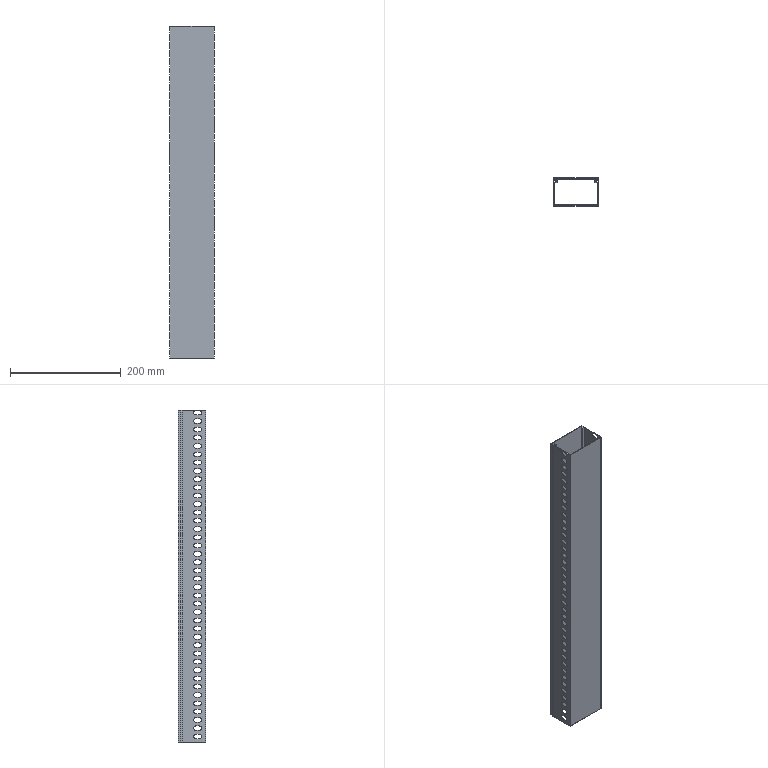Part | SolidWorks | features BaseBody 1 | 1 solid | 346 faces | box 80 x 50 x 600 mm | volume 157739 mm3 | plane 186 | cylinder 160 | commonest cylinder face diameters 8 x160